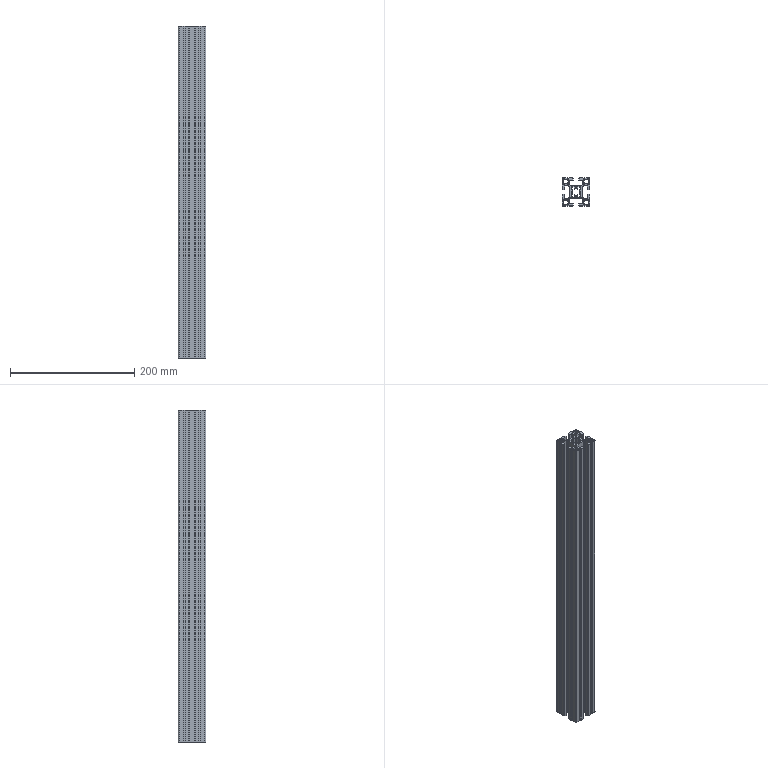Part | STEP file | 4545 profile 2 | 1 solid | 262 faces | box 45 x 45 x 535 mm | volume 371208 mm3 | plane 186 | cylinder 76 | commonest cylinder face diameters 2 x44 8 x20 12 x8 4 x4